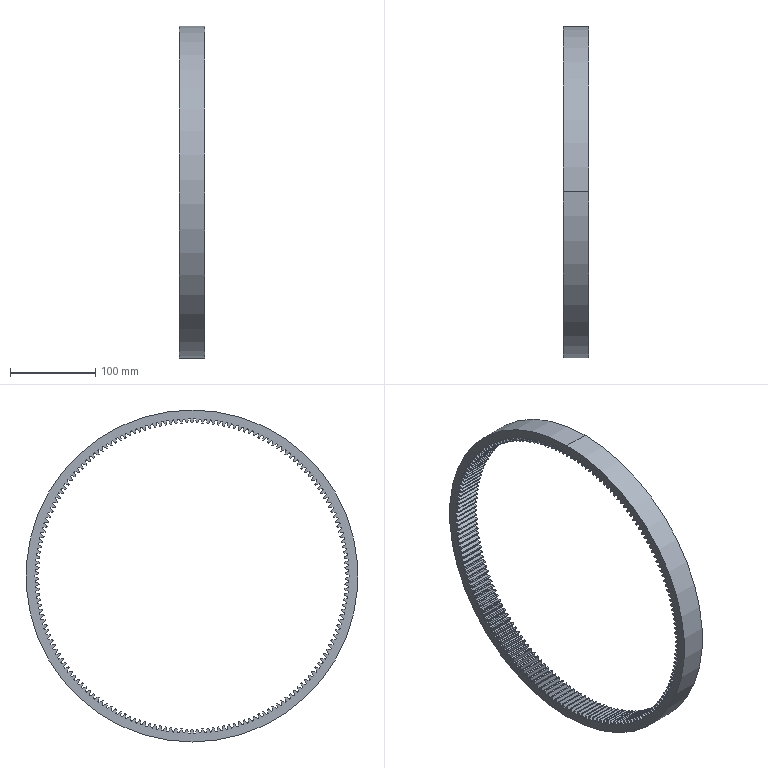Part | SolidWorks | features ICE 1, MBimport 1, MoveFace 1 | 1 solid | 737 faces | box 30 x 390 x 390 mm | volume 449494 mm3 | cylinder 735 | plane 2 | commonest cylinder face diameters 182 x368 360 x183 369.002 x182 390 x2